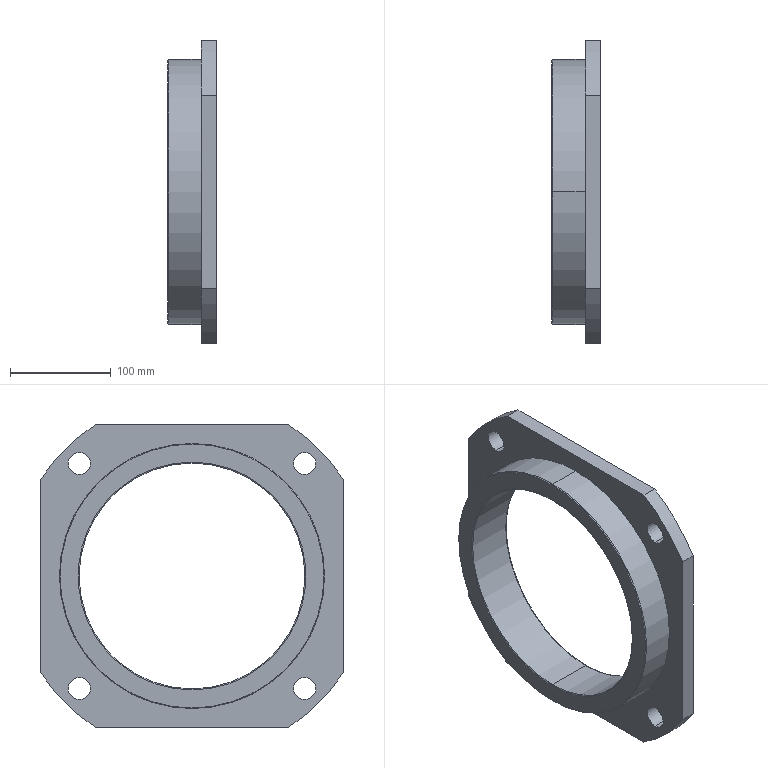Part | SolidWorks | features Chamfer 3, ICE 2, CirPattern 1, RefAxis 1, Revolution 1 | 1 solid | 29 faces | box 48 x 300 x 300 mm | volume 1152473 mm3 | cylinder 16 | plane 7 | cone 6 | commonest cylinder face diameters 22 x8 356 x4 224 x2 263 x2
STEP:
#1=CARTESIAN_POINT('',(-36.947,0.,130.923));
#2=VERTEX_POINT('',#1);
#3=CARTESIAN_POINT('',(-36.947,0.,-130.923));
#4=VERTEX_POINT('',#3);
#5=CARTESIAN_POINT('',(-36.947,0.,0.));
#6=DIRECTION('',(-1.,0.,0.));
#7=DIRECTION('',(0.,0.,-1.));
#8=AXIS2_PLACEMENT_3D('',#5,#6,#7);
#9=CIRCLE('',#8,130.923);
#10=EDGE_CURVE('',#2,#4,#9,.T.);
#11=ORIENTED_EDGE('',*,*,#10,.F.);
#12=CARTESIAN_POINT('',(-35.947,0.,131.5));
#13=VERTEX_POINT('',#12);
#14=CARTESIAN_POINT('',(-36.947,0.,130.923));
#15=DIRECTION('',(0.866,0.,0.5));
#16=VECTOR('',#15,1000.);
#17=LINE('',#14,#16);
#18=EDGE_CURVE('',#2,#13,#17,.T.);
#19=ORIENTED_EDGE('',*,*,#18,.T.);
#20=CARTESIAN_POINT('',(-35.947,0.,-131.5));
#21=VERTEX_POINT('',#20);
#22=CARTESIAN_POINT('',(-35.947,0.,0.));
#23=DIRECTION('',(1.,0.,0.));
#24=DIRECTION('',(0.,0.,-1.));
#25=AXIS2_PLACEMENT_3D('',#22,#23,#24);
#26=CIRCLE('',#25,131.5);
#27=EDGE_CURVE('',#21,#13,#26,.T.);
#28=ORIENTED_EDGE('',*,*,#27,.F.);
#29=CARTESIAN_POINT('',(-36.947,0.,-130.923));
#30=DIRECTION('',(0.866,0.,-0.5));
#31=VECTOR('',#30,1000.);
#32=LINE('',#29,#31);
#33=EDGE_CURVE('',#4,#21,#32,.T.);
#34=ORIENTED_EDGE('',*,*,#33,.F.);
#35=EDGE_LOOP('',(#11,#19,#28,#34));
#36=FACE_OUTER_BOUND('',#35,.T.);
#37=CARTESIAN_POINT('',(-36.947,0.,0.));
#38=DIRECTION('',(1.,0.,0.));
#39=DIRECTION('',(0.,0.,-1.));
#40=AXIS2_PLACEMENT_3D('',#37,#38,#39);
#41=CONICAL_SURFACE('',#40,130.923,0.5236);
#42=ADVANCED_FACE('',(#36),#41,.T.);
#43=CARTESIAN_POINT('',(-36.37,0.,-112.));
#44=VERTEX_POINT('',#43);
#45=CARTESIAN_POINT('',(-36.37,0.,112.));
#46=VERTEX_POINT('',#45);
#47=CARTESIAN_POINT('',(-36.37,0.,0.));
#48=DIRECTION('',(-1.,0.,0.));
#49=DIRECTION('',(0.,0.,-1.));
#50=AXIS2_PLACEMENT_3D('',#47,#48,#49);
#51=CIRCLE('',#50,112.);
#52=EDGE_CURVE('',#44,#46,#51,.T.);
#53=ORIENTED_EDGE('',*,*,#52,.F.);
#54=CARTESIAN_POINT('',(-36.947,0.,-113.));
#55=VERTEX_POINT('',#54);
#56=CARTESIAN_POINT('',(-36.37,0.,-112.));
#57=DIRECTION('',(-0.5,0.,-0.866));
#58=VECTOR('',#57,1000.);
#59=LINE('',#56,#58);
#60=EDGE_CURVE('',#44,#55,#59,.T.);
#61=ORIENTED_EDGE('',*,*,#60,.T.);
#62=CARTESIAN_POINT('',(-36.947,0.,113.));
#63=VERTEX_POINT('',#62);
#64=CARTESIAN_POINT('',(-36.947,0.,0.));
#65=DIRECTION('',(1.,0.,0.));
#66=DIRECTION('',(0.,0.,-1.));
#67=AXIS2_PLACEMENT_3D('',#64,#65,#66);
#68=CIRCLE('',#67,113.);
#69=EDGE_CURVE('',#63,#55,#68,.T.);
#70=ORIENTED_EDGE('',*,*,#69,.F.);
#71=CARTESIAN_POINT('',(-36.37,0.,112.));
#72=DIRECTION('',(-0.5,0.,0.866));
#73=VECTOR('',#72,1000.);
#74=LINE('',#71,#73);
#75=EDGE_CURVE('',#46,#63,#74,.T.);
#76=ORIENTED_EDGE('',*,*,#75,.F.);
#77=EDGE_LOOP('',(#53,#61,#70,#76));
#78=FACE_OUTER_BOUND('',#77,.T.);
#79=CARTESIAN_POINT('',(-36.37,0.,0.));
#80=DIRECTION('',(-1.,0.,0.));
#81=DIRECTION('',(0.,0.,1.));
#82=AXIS2_PLACEMENT_3D('',#79,#80,#81);
#83=CONICAL_SURFACE('',#82,112.,1.047);
#84=ADVANCED_FACE('',(#78),#83,.F.);
#85=CARTESIAN_POINT('',(10.053,0.,112.));
#86=VERTEX_POINT('',#85);
#87=CARTESIAN_POINT('',(10.053,0.,-112.));
#88=VERTEX_POINT('',#87);
#89=CARTESIAN_POINT('',(10.053,0.,0.));
#90=DIRECTION('',(1.,0.,0.));
#91=DIRECTION('',(0.,0.,1.));
#92=AXIS2_PLACEMENT_3D('',#89,#90,#91);
#93=CIRCLE('',#92,112.);
#94=EDGE_CURVE('',#86,#88,#93,.T.);
#95=ORIENTED_EDGE('',*,*,#94,.F.);
#96=CARTESIAN_POINT('',(11.053,0.,112.577));
#97=VERTEX_POINT('',#96);
#98=CARTESIAN_POINT('',(11.053,0.,112.577));
#99=DIRECTION('',(0.866,0.,0.5));
#100=VECTOR('',#99,1000.);
#101=LINE('',#98,#100);
#102=EDGE_CURVE('',#86,#97,#101,.T.);
#103=ORIENTED_EDGE('',*,*,#102,.T.);
#104=CARTESIAN_POINT('',(11.053,0.,-112.577));
#105=VERTEX_POINT('',#104);
#106=CARTESIAN_POINT('',(11.053,0.,0.));
#107=DIRECTION('',(-1.,0.,0.));
#108=DIRECTION('',(0.,0.,1.));
#109=AXIS2_PLACEMENT_3D('',#106,#107,#108);
#110=CIRCLE('',#109,112.577);
#111=EDGE_CURVE('',#105,#97,#110,.T.);
#112=ORIENTED_EDGE('',*,*,#111,.F.);
#113=CARTESIAN_POINT('',(11.053,0.,-112.577));
#114=DIRECTION('',(0.866,0.,-0.5));
#115=VECTOR('',#114,1000.);
#116=LINE('',#113,#115);
#117=EDGE_CURVE('',#88,#105,#116,.T.);
#118=ORIENTED_EDGE('',*,*,#117,.F.);
#119=EDGE_LOOP('',(#95,#103,#112,#118));
#120=FACE_OUTER_BOUND('',#119,.T.);
#121=CARTESIAN_POINT('',(11.053,0.,0.));
#122=DIRECTION('',(1.,0.,0.));
#123=DIRECTION('',(0.,0.,-1.));
#124=AXIS2_PLACEMENT_3D('',#121,#122,#123);
#125=CONICAL_SURFACE('',#124,112.577,0.5236);
#126=ADVANCED_FACE('',(#120),#125,.F.);
#127=CARTESIAN_POINT('',(-3.947,111.723,122.723));
#128=VERTEX_POINT('',#127);
#129=CARTESIAN_POINT('',(-3.947,111.723,100.723));
#130=VERTEX_POINT('',#129);
#131=CARTESIAN_POINT('',(-3.947,111.723,111.723));
#132=DIRECTION('',(1.,0.,0.));
#133=DIRECTION('',(0.,1.,0.));
#134=AXIS2_PLACEMENT_3D('',#131,#132,#133);
#135=CIRCLE('',#134,11.);
#136=EDGE_CURVE('',#128,#130,#135,.T.);
#137=ORIENTED_EDGE('',*,*,#136,.F.);
#138=CARTESIAN_POINT('',(11.053,111.723,122.723));
#139=VERTEX_POINT('',#138);
#140=CARTESIAN_POINT('',(-3.947,111.723,122.723));
#141=DIRECTION('',(1.,0.,0.));
#142=VECTOR('',#141,1000.);
#143=LINE('',#140,#142);
#144=EDGE_CURVE('',#128,#139,#143,.T.);
#145=ORIENTED_EDGE('',*,*,#144,.T.);
#146=CARTESIAN_POINT('',(11.053,111.723,100.723));
#147=VERTEX_POINT('',#146);
#148=CARTESIAN_POINT('',(11.053,111.723,111.723));
#149=DIRECTION('',(1.,0.,0.));
#150=DIRECTION('',(0.,1.,0.));
#151=AXIS2_PLACEMENT_3D('',#148,#149,#150);
#152=CIRCLE('',#151,11.);
#153=EDGE_CURVE('',#139,#147,#152,.T.);
#154=ORIENTED_EDGE('',*,*,#153,.T.);
#155=CARTESIAN_POINT('',(-3.947,111.723,100.723));
#156=DIRECTION('',(1.,0.,0.));
#157=VECTOR('',#156,1000.);
#158=LINE('',#155,#157);
#159=EDGE_CURVE('',#130,#147,#158,.T.);
#160=ORIENTED_EDGE('',*,*,#159,.F.);
#161=EDGE_LOOP('',(#137,#145,#154,#160));
#162=FACE_OUTER_BOUND('',#161,.T.);
#163=CARTESIAN_POINT('',(-3.947,111.723,111.723));
#164=DIRECTION('',(1.,0.,0.));
#165=DIRECTION('',(0.,0.,-1.));
#166=AXIS2_PLACEMENT_3D('',#163,#164,#165);
#167=CYLINDRICAL_SURFACE('',#166,11.);
#168=ADVANCED_FACE('',(#162),#167,.F.);
#169=CARTESIAN_POINT('',(-3.947,-111.723,122.723));
#170=VERTEX_POINT('',#169);
#171=CARTESIAN_POINT('',(-3.947,-111.723,100.723));
#172=VERTEX_POINT('',#171);
#173=CARTESIAN_POINT('',(-3.947,-111.723,111.723));
#174=DIRECTION('',(1.,0.,0.));
#175=DIRECTION('',(0.,0.,1.));
#176=AXIS2_PLACEMENT_3D('',#173,#174,#175);
#177=CIRCLE('',#176,11.);
#178=EDGE_CURVE('',#170,#172,#177,.T.);
#179=ORIENTED_EDGE('',*,*,#178,.F.);
#180=CARTESIAN_POINT('',(11.053,-111.723,122.723));
#181=VERTEX_POINT('',#180);
#182=CARTESIAN_POINT('',(-3.947,-111.723,122.723));
#183=DIRECTION('',(1.,0.,0.));
#184=VECTOR('',#183,1000.);
#185=LINE('',#182,#184);
#186=EDGE_CURVE('',#170,#181,#185,.T.);
#187=ORIENTED_EDGE('',*,*,#186,.T.);
#188=CARTESIAN_POINT('',(11.053,-111.723,100.723));
#189=VERTEX_POINT('',#188);
#190=CARTESIAN_POINT('',(11.053,-111.723,111.723));
#191=DIRECTION('',(1.,0.,0.));
#192=DIRECTION('',(0.,0.,1.));
#193=AXIS2_PLACEMENT_3D('',#190,#191,#192);
#194=CIRCLE('',#193,11.);
#195=EDGE_CURVE('',#181,#189,#194,.T.);
#196=ORIENTED_EDGE('',*,*,#195,.T.);
#197=CARTESIAN_POINT('',(-3.947,-111.723,100.723));
#198=DIRECTION('',(1.,0.,0.));
#199=VECTOR('',#198,1000.);
#200=LINE('',#197,#199);
#201=EDGE_CURVE('',#172,#189,#200,.T.);
#202=ORIENTED_EDGE('',*,*,#201,.F.);
#203=EDGE_LOOP('',(#179,#187,#196,#202));
#204=FACE_OUTER_BOUND('',#203,.T.);
#205=CARTESIAN_POINT('',(-3.947,-111.723,111.723));
#206=DIRECTION('',(1.,0.,0.));
#207=DIRECTION('',(0.,0.,-1.));
#208=AXIS2_PLACEMENT_3D('',#205,#206,#207);
#209=CYLINDRICAL_SURFACE('',#208,11.);
#210=ADVANCED_FACE('',(#204),#209,.F.);
#211=CARTESIAN_POINT('',(-3.947,-111.723,-100.723));
#212=VERTEX_POINT('',#211);
#213=CARTESIAN_POINT('',(-3.947,-111.723,-122.723));
#214=VERTEX_POINT('',#213);
#215=CARTESIAN_POINT('',(-3.947,-111.723,-111.723));
#216=DIRECTION('',(1.,0.,0.));
#217=DIRECTION('',(0.,-1.,0.));
#218=AXIS2_PLACEMENT_3D('',#215,#216,#217);
#219=CIRCLE('',#218,11.);
#220=EDGE_CURVE('',#212,#214,#219,.T.);
#221=ORIENTED_EDGE('',*,*,#220,.F.);
#222=CARTESIAN_POINT('',(11.053,-111.723,-100.723));
#223=VERTEX_POINT('',#222);
#224=CARTESIAN_POINT('',(-3.947,-111.723,-100.723));
#225=DIRECTION('',(1.,0.,0.));
#226=VECTOR('',#225,1000.);
#227=LINE('',#224,#226);
#228=EDGE_CURVE('',#212,#223,#227,.T.);
#229=ORIENTED_EDGE('',*,*,#228,.T.);
#230=CARTESIAN_POINT('',(11.053,-111.723,-122.723));
#231=VERTEX_POINT('',#230);
#232=CARTESIAN_POINT('',(11.053,-111.723,-111.723));
#233=DIRECTION('',(1.,0.,0.));
#234=DIRECTION('',(0.,-1.,0.));
#235=AXIS2_PLACEMENT_3D('',#232,#233,#234);
#236=CIRCLE('',#235,11.);
#237=EDGE_CURVE('',#223,#231,#236,.T.);
#238=ORIENTED_EDGE('',*,*,#237,.T.);
#239=CARTESIAN_POINT('',(-3.947,-111.723,-122.723));
#240=DIRECTION('',(1.,0.,0.));
#241=VECTOR('',#240,1000.);
#242=LINE('',#239,#241);
#243=EDGE_CURVE('',#214,#231,#242,.T.);
#244=ORIENTED_EDGE('',*,*,#243,.F.);
#245=EDGE_LOOP('',(#221,#229,#238,#244));
#246=FACE_OUTER_BOUND('',#245,.T.);
#247=CARTESIAN_POINT('',(-3.947,-111.723,-111.723));
#248=DIRECTION('',(1.,0.,0.));
#249=DIRECTION('',(0.,0.,-1.));
#250=AXIS2_PLACEMENT_3D('',#247,#248,#249);
#251=CYLINDRICAL_SURFACE('',#250,11.);
#252=ADVANCED_FACE('',(#246),#251,.F.);
#253=CARTESIAN_POINT('',(-3.947,111.723,-100.723));
#254=VERTEX_POINT('',#253);
#255=CARTESIAN_POINT('',(-3.947,111.723,-122.723));
#256=VERTEX_POINT('',#255);
#257=CARTESIAN_POINT('',(-3.947,111.723,-111.723));
#258=DIRECTION('',(1.,0.,0.));
#259=DIRECTION('',(0.,0.,-1.));
#260=AXIS2_PLACEMENT_3D('',#257,#258,#259);
#261=CIRCLE('',#260,11.);
#262=EDGE_CURVE('',#254,#256,#261,.T.);
#263=ORIENTED_EDGE('',*,*,#262,.F.);
#264=CARTESIAN_POINT('',(11.053,111.723,-100.723));
#265=VERTEX_POINT('',#264);
#266=CARTESIAN_POINT('',(-3.947,111.723,-100.723));
#267=DIRECTION('',(1.,0.,0.));
#268=VECTOR('',#267,1000.);
#269=LINE('',#266,#268);
#270=EDGE_CURVE('',#254,#265,#269,.T.);
#271=ORIENTED_EDGE('',*,*,#270,.T.);
#272=CARTESIAN_POINT('',(11.053,111.723,-122.723));
#273=VERTEX_POINT('',#272);
#274=CARTESIAN_POINT('',(11.053,111.723,-111.723));
#275=DIRECTION('',(1.,0.,0.));
#276=DIRECTION('',(0.,0.,-1.));
#277=AXIS2_PLACEMENT_3D('',#274,#275,#276);
#278=CIRCLE('',#277,11.);
#279=EDGE_CURVE('',#265,#273,#278,.T.);
#280=ORIENTED_EDGE('',*,*,#279,.T.);
#281=CARTESIAN_POINT('',(-3.947,111.723,-122.723));
#282=DIRECTION('',(1.,0.,0.));
#283=VECTOR('',#282,1000.);
#284=LINE('',#281,#283);
#285=EDGE_CURVE('',#256,#273,#284,.T.);
#286=ORIENTED_EDGE('',*,*,#285,.F.);
#287=EDGE_LOOP('',(#263,#271,#280,#286));
#288=FACE_OUTER_BOUND('',#287,.T.);
#289=CARTESIAN_POINT('',(-3.947,111.723,-111.723));
#290=DIRECTION('',(1.,0.,0.));
#291=DIRECTION('',(0.,0.,-1.));
#292=AXIS2_PLACEMENT_3D('',#289,#290,#291);
#293=CYLINDRICAL_SURFACE('',#292,11.);
#294=ADVANCED_FACE('',(#288),#293,.F.);
#295=ORIENTED_EDGE('',*,*,#94,.T.);
#296=CARTESIAN_POINT('',(-77.414,0.,-112.));
#297=DIRECTION('',(-1.,0.,0.));
#298=VECTOR('',#297,1000.);
#299=LINE('',#296,#298);
#300=EDGE_CURVE('',#88,#44,#299,.T.);
#301=ORIENTED_EDGE('',*,*,#300,.T.);
#302=ORIENTED_EDGE('',*,*,#52,.T.);
#303=CARTESIAN_POINT('',(-77.414,0.,112.));
#304=DIRECTION('',(-1.,0.,0.));
#305=VECTOR('',#304,1000.);
#306=LINE('',#303,#305);
#307=EDGE_CURVE('',#86,#46,#306,.T.);
#308=ORIENTED_EDGE('',*,*,#307,.F.);
#309=EDGE_LOOP('',(#295,#301,#302,#308));
#310=FACE_OUTER_BOUND('',#309,.T.);
#311=CARTESIAN_POINT('',(-77.414,0.,0.));
#312=DIRECTION('',(-1.,0.,0.));
#313=DIRECTION('',(0.,0.,1.));
#314=AXIS2_PLACEMENT_3D('',#311,#312,#313);
#315=CYLINDRICAL_SURFACE('',#314,112.);
#316=ADVANCED_FACE('',(#310),#315,.F.);
#317=CARTESIAN_POINT('',(-3.947,0.,131.5));
#318=VERTEX_POINT('',#317);
#319=CARTESIAN_POINT('',(-3.947,0.,-131.5));
#320=VERTEX_POINT('',#319);
#321=CARTESIAN_POINT('',(-3.947,0.,0.));
#322=DIRECTION('',(-1.,0.,0.));
#323=DIRECTION('',(0.,0.,1.));
#324=AXIS2_PLACEMENT_3D('',#321,#322,#323);
#325=CIRCLE('',#324,131.5);
#326=EDGE_CURVE('',#318,#320,#325,.T.);
#327=ORIENTED_EDGE('',*,*,#326,.T.);
#328=CARTESIAN_POINT('',(-77.414,0.,-131.5));
#329=DIRECTION('',(-1.,0.,0.));
#330=VECTOR('',#329,1000.);
#331=LINE('',#328,#330);
#332=EDGE_CURVE('',#320,#21,#331,.T.);
#333=ORIENTED_EDGE('',*,*,#332,.T.);
#334=ORIENTED_EDGE('',*,*,#27,.T.);
#335=CARTESIAN_POINT('',(-77.414,0.,131.5));
#336=DIRECTION('',(-1.,0.,0.));
#337=VECTOR('',#336,1000.);
#338=LINE('',#335,#337);
#339=EDGE_CURVE('',#318,#13,#338,.T.);
#340=ORIENTED_EDGE('',*,*,#339,.F.);
#341=EDGE_LOOP('',(#327,#333,#334,#340));
#342=FACE_OUTER_BOUND('',#341,.T.);
#343=CARTESIAN_POINT('',(-77.414,0.,0.));
#344=DIRECTION('',(-1.,0.,0.));
#345=DIRECTION('',(0.,0.,1.));
#346=AXIS2_PLACEMENT_3D('',#343,#344,#345);
#347=CYLINDRICAL_SURFACE('',#346,131.5);
#348=ADVANCED_FACE('',(#342),#347,.T.);
#349=CARTESIAN_POINT('',(11.053,-150.,95.833));
#350=VERTEX_POINT('',#349);
#351=CARTESIAN_POINT('',(11.053,-95.833,150.));
#352=VERTEX_POINT('',#351);
#353=CARTESIAN_POINT('',(11.053,0.,0.));
#354=DIRECTION('',(-1.,0.,0.));
#355=DIRECTION('',(0.,0.,1.));
#356=AXIS2_PLACEMENT_3D('',#353,#354,#355);
#357=CIRCLE('',#356,178.);
#358=EDGE_CURVE('',#350,#352,#357,.T.);
#359=ORIENTED_EDGE('',*,*,#358,.T.);
#360=CARTESIAN_POINT('',(-3.947,-95.833,150.));
#361=VERTEX_POINT('',#360);
#362=CARTESIAN_POINT('',(-3.947,-95.833,150.));
#363=DIRECTION('',(1.,0.,0.));
#364=VECTOR('',#363,1000.);
#365=LINE('',#362,#364);
#366=EDGE_CURVE('',#361,#352,#365,.T.);
#367=ORIENTED_EDGE('',*,*,#366,.F.);
#368=CARTESIAN_POINT('',(-3.947,-150.,95.833));
#369=VERTEX_POINT('',#368);
#370=CARTESIAN_POINT('',(-3.947,0.,0.));
#371=DIRECTION('',(-1.,0.,0.));
#372=DIRECTION('',(0.,0.,1.));
#373=AXIS2_PLACEMENT_3D('',#370,#371,#372);
#374=CIRCLE('',#373,178.);
#375=EDGE_CURVE('',#369,#361,#374,.T.);
#376=ORIENTED_EDGE('',*,*,#375,.F.);
#377=CARTESIAN_POINT('',(-3.947,-150.,95.833));
#378=DIRECTION('',(1.,0.,0.));
#379=VECTOR('',#378,1000.);
#380=LINE('',#377,#379);
#381=EDGE_CURVE('',#369,#350,#380,.T.);
#382=ORIENTED_EDGE('',*,*,#381,.T.);
#383=EDGE_LOOP('',(#359,#367,#376,#382));
#384=FACE_OUTER_BOUND('',#383,.T.);
#385=CARTESIAN_POINT('',(-77.414,0.,0.));
#386=DIRECTION('',(-1.,0.,0.));
#387=DIRECTION('',(0.,0.,1.));
#388=AXIS2_PLACEMENT_3D('',#385,#386,#387);
#389=CYLINDRICAL_SURFACE('',#388,178.);
#390=ADVANCED_FACE('',(#384),#389,.T.);
#391=CARTESIAN_POINT('',(-3.947,95.833,150.));
#392=VERTEX_POINT('',#391);
#393=CARTESIAN_POINT('',(-3.947,150.,95.833));
#394=VERTEX_POINT('',#393);
#395=CARTESIAN_POINT('',(-3.947,0.,0.));
#396=DIRECTION('',(-1.,0.,0.));
#397=DIRECTION('',(0.,0.,1.));
#398=AXIS2_PLACEMENT_3D('',#395,#396,#397);
#399=CIRCLE('',#398,178.);
#400=EDGE_CURVE('',#392,#394,#399,.T.);
#401=ORIENTED_EDGE('',*,*,#400,.F.);
#402=CARTESIAN_POINT('',(11.053,95.833,150.));
#403=VERTEX_POINT('',#402);
#404=CARTESIAN_POINT('',(-3.947,95.833,150.));
#405=DIRECTION('',(1.,0.,0.));
#406=VECTOR('',#405,1000.);
#407=LINE('',#404,#406);
#408=EDGE_CURVE('',#392,#403,#407,.T.);
#409=ORIENTED_EDGE('',*,*,#408,.T.);
#410=CARTESIAN_POINT('',(11.053,150.,95.833));
#411=VERTEX_POINT('',#410);
#412=CARTESIAN_POINT('',(11.053,0.,0.));
#413=DIRECTION('',(-1.,0.,0.));
#414=DIRECTION('',(0.,0.,1.));
#415=AXIS2_PLACEMENT_3D('',#412,#413,#414);
#416=CIRCLE('',#415,178.);
#417=EDGE_CURVE('',#403,#411,#416,.T.);
#418=ORIENTED_EDGE('',*,*,#417,.T.);
#419=CARTESIAN_POINT('',(-3.947,150.,95.833));
#420=DIRECTION('',(1.,0.,0.));
#421=VECTOR('',#420,1000.);
#422=LINE('',#419,#421);
#423=EDGE_CURVE('',#394,#411,#422,.T.);
#424=ORIENTED_EDGE('',*,*,#423,.F.);
#425=EDGE_LOOP('',(#401,#409,#418,#424));
#426=FACE_OUTER_BOUND('',#425,.T.);
#427=CARTESIAN_POINT('',(-77.414,0.,0.));
#428=DIRECTION('',(-1.,0.,0.));
#429=DIRECTION('',(0.,0.,1.));
#430=AXIS2_PLACEMENT_3D('',#427,#428,#429);
#431=CYLINDRICAL_SURFACE('',#430,178.);
#432=ADVANCED_FACE('',(#426),#431,.T.);
#433=CARTESIAN_POINT('',(11.053,-95.833,-150.));
#434=VERTEX_POINT('',#433);
#435=CARTESIAN_POINT('',(11.053,-150.,-95.833));
#436=VERTEX_POINT('',#435);
#437=CARTESIAN_POINT('',(11.053,0.,0.));
#438=DIRECTION('',(-1.,0.,0.));
#439=DIRECTION('',(0.,0.,1.));
#440=AXIS2_PLACEMENT_3D('',#437,#438,#439);
#441=CIRCLE('',#440,178.);
#442=EDGE_CURVE('',#434,#436,#441,.T.);
#443=ORIENTED_EDGE('',*,*,#442,.T.);
#444=CARTESIAN_POINT('',(-3.947,-150.,-95.833));
#445=VERTEX_POINT('',#444);
#446=CARTESIAN_POINT('',(-3.947,-150.,-95.833));
#447=DIRECTION('',(1.,0.,0.));
#448=VECTOR('',#447,1000.);
#449=LINE('',#446,#448);
#450=EDGE_CURVE('',#445,#436,#449,.T.);
#451=ORIENTED_EDGE('',*,*,#450,.F.);
#452=CARTESIAN_POINT('',(-3.947,-95.833,-150.));
#453=VERTEX_POINT('',#452);
#454=CARTESIAN_POINT('',(-3.947,0.,0.));
#455=DIRECTION('',(-1.,0.,0.));
#456=DIRECTION('',(0.,0.,1.));
#457=AXIS2_PLACEMENT_3D('',#454,#455,#456);
#458=CIRCLE('',#457,178.);
#459=EDGE_CURVE('',#453,#445,#458,.T.);
#460=ORIENTED_EDGE('',*,*,#459,.F.);
#461=CARTESIAN_POINT('',(-3.947,-95.833,-150.));
#462=DIRECTION('',(1.,0.,0.));
#463=VECTOR('',#462,1000.);
#464=LINE('',#461,#463);
#465=EDGE_CURVE('',#453,#434,#464,.T.);
#466=ORIENTED_EDGE('',*,*,#465,.T.);
#467=EDGE_LOOP('',(#443,#451,#460,#466));
#468=FACE_OUTER_BOUND('',#467,.T.);
#469=CARTESIAN_POINT('',(-77.414,0.,0.));
#470=DIRECTION('',(-1.,0.,0.));
#471=DIRECTION('',(0.,0.,1.));
#472=AXIS2_PLACEMENT_3D('',#469,#470,#471);
#473=CYLINDRICAL_SURFACE('',#472,178.);
#474=ADVANCED_FACE('',(#468),#473,.T.);
#475=CARTESIAN_POINT('',(-36.947,0.,0.));
#476=DIRECTION('',(-1.,0.,0.));
#477=DIRECTION('',(0.,0.,-1.));
#478=AXIS2_PLACEMENT_3D('',#475,#476,#477);
#479=CIRCLE('',#478,130.923);
#480=EDGE_CURVE('',#4,#2,#479,.T.);
#481=ORIENTED_EDGE('',*,*,#480,.T.);
#482=ORIENTED_EDGE('',*,*,#10,.T.);
#483=EDGE_LOOP('',(#481,#482));
#484=FACE_OUTER_BOUND('',#483,.T.);
#485=ORIENTED_EDGE('',*,*,#69,.T.);
#486=CARTESIAN_POINT('',(-36.947,0.,0.));
#487=DIRECTION('',(1.,0.,0.));
#488=DIRECTION('',(0.,0.,-1.));
#489=AXIS2_PLACEMENT_3D('',#486,#487,#488);
#490=CIRCLE('',#489,113.);
#491=EDGE_CURVE('',#55,#63,#490,.T.);
#492=ORIENTED_EDGE('',*,*,#491,.T.);
#493=EDGE_LOOP('',(#485,#492));
#494=FACE_BOUND('',#493,.T.);
#495=CARTESIAN_POINT('',(-36.947,112.,0.));
#496=DIRECTION('',(1.,0.,0.));
#497=DIRECTION('',(0.,0.,-1.));
#498=AXIS2_PLACEMENT_3D('',#495,#496,#497);
#499=PLANE('',#498);
#500=ADVANCED_FACE('',(#484,#494),#499,.F.);
#501=ORIENTED_EDGE('',*,*,#332,.F.);
#502=CARTESIAN_POINT('',(-3.947,0.,0.));
#503=DIRECTION('',(-1.,0.,0.));
#504=DIRECTION('',(0.,0.,1.));
#505=AXIS2_PLACEMENT_3D('',#502,#503,#504);
#506=CIRCLE('',#505,131.5);
#507=EDGE_CURVE('',#320,#318,#506,.T.);
#508=ORIENTED_EDGE('',*,*,#507,.T.);
#509=ORIENTED_EDGE('',*,*,#339,.T.);
#510=CARTESIAN_POINT('',(-35.947,0.,0.));
#511=DIRECTION('',(1.,0.,0.));
#512=DIRECTION('',(0.,0.,-1.));
#513=AXIS2_PLACEMENT_3D('',#510,#511,#512);
#514=CIRCLE('',#513,131.5);
#515=EDGE_CURVE('',#13,#21,#514,.T.);
#516=ORIENTED_EDGE('',*,*,#515,.T.);
#517=EDGE_LOOP('',(#501,#508,#509,#516));
#518=FACE_OUTER_BOUND('',#517,.T.);
#519=CARTESIAN_POINT('',(-77.414,0.,0.));
#520=DIRECTION('',(-1.,0.,0.));
#521=DIRECTION('',(0.,0.,1.));
#522=AXIS2_PLACEMENT_3D('',#519,#520,#521);
#523=CYLINDRICAL_SURFACE('',#522,131.5);
#524=ADVANCED_FACE('',(#518),#523,.T.);
#525=CARTESIAN_POINT('',(-3.947,111.723,111.723));
#526=DIRECTION('',(1.,0.,0.));
#527=DIRECTION('',(0.,1.,0.));
#528=AXIS2_PLACEMENT_3D('',#525,#526,#527);
#529=CIRCLE('',#528,11.);
#530=EDGE_CURVE('',#130,#128,#529,.T.);
#531=ORIENTED_EDGE('',*,*,#530,.T.);
#532=ORIENTED_EDGE('',*,*,#136,.T.);
#533=EDGE_LOOP('',(#531,#532));
#534=FACE_BOUND('',#533,.T.);
#535=CARTESIAN_POINT('',(-3.947,-111.723,111.723));
#536=DIRECTION('',(1.,0.,0.));
#537=DIRECTION('',(0.,0.,1.));
#538=AXIS2_PLACEMENT_3D('',#535,#536,#537);
#539=CIRCLE('',#538,11.);
#540=EDGE_CURVE('',#172,#170,#539,.T.);
#541=ORIENTED_EDGE('',*,*,#540,.T.);
#542=ORIENTED_EDGE('',*,*,#178,.T.);
#543=EDGE_LOOP('',(#541,#542));
#544=FACE_BOUND('',#543,.T.);
#545=CARTESIAN_POINT('',(-3.947,-111.723,-111.723));
#546=DIRECTION('',(1.,0.,0.));
#547=DIRECTION('',(0.,-1.,0.));
#548=AXIS2_PLACEMENT_3D('',#545,#546,#547);
#549=CIRCLE('',#548,11.);
#550=EDGE_CURVE('',#214,#212,#549,.T.);
#551=ORIENTED_EDGE('',*,*,#550,.T.);
#552=ORIENTED_EDGE('',*,*,#220,.T.);
#553=EDGE_LOOP('',(#551,#552));
#554=FACE_BOUND('',#553,.T.);
#555=CARTESIAN_POINT('',(-3.947,111.723,-111.723));
#556=DIRECTION('',(1.,0.,0.));
#557=DIRECTION('',(0.,0.,-1.));
#558=AXIS2_PLACEMENT_3D('',#555,#556,#557);
#559=CIRCLE('',#558,11.);
#560=EDGE_CURVE('',#256,#254,#559,.T.);
#561=ORIENTED_EDGE('',*,*,#560,.T.);
#562=ORIENTED_EDGE('',*,*,#262,.T.);
#563=EDGE_LOOP('',(#561,#562));
#564=FACE_BOUND('',#563,.T.);
#565=ORIENTED_EDGE('',*,*,#326,.F.);
#566=ORIENTED_EDGE('',*,*,#507,.F.);
#567=EDGE_LOOP('',(#565,#566));
#568=FACE_BOUND('',#567,.T.);
#569=ORIENTED_EDGE('',*,*,#375,.T.);
#570=CARTESIAN_POINT('',(-3.947,95.833,150.));
#571=DIRECTION('',(0.,1.,0.));
#572=VECTOR('',#571,1000.);
#573=LINE('',#570,#572);
#574=EDGE_CURVE('',#361,#392,#573,.T.);
#575=ORIENTED_EDGE('',*,*,#574,.T.);
#576=ORIENTED_EDGE('',*,*,#400,.T.);
#577=CARTESIAN_POINT('',(-3.947,150.,-95.833));
#578=VERTEX_POINT('',#577);
#579=CARTESIAN_POINT('',(-3.947,150.,95.833));
#580=DIRECTION('',(0.,0.,-1.));
#581=VECTOR('',#580,1000.);
#582=LINE('',#579,#581);
#583=EDGE_CURVE('',#394,#578,#582,.T.);
#584=ORIENTED_EDGE('',*,*,#583,.T.);
#585=CARTESIAN_POINT('',(-3.947,95.833,-150.));
#586=VERTEX_POINT('',#585);
#587=CARTESIAN_POINT('',(-3.947,0.,0.));
#588=DIRECTION('',(-1.,0.,0.));
#589=DIRECTION('',(0.,0.,1.));
#590=AXIS2_PLACEMENT_3D('',#587,#588,#589);
#591=CIRCLE('',#590,178.);
#592=EDGE_CURVE('',#578,#586,#591,.T.);
#593=ORIENTED_EDGE('',*,*,#592,.T.);
#594=CARTESIAN_POINT('',(-3.947,95.833,-150.));
#595=DIRECTION('',(0.,-1.,0.));
#596=VECTOR('',#595,1000.);
#597=LINE('',#594,#596);
#598=EDGE_CURVE('',#586,#453,#597,.T.);
#599=ORIENTED_EDGE('',*,*,#598,.T.);
#600=ORIENTED_EDGE('',*,*,#459,.T.);
#601=CARTESIAN_POINT('',(-3.947,-150.,95.833));
#602=DIRECTION('',(0.,0.,1.));
#603=VECTOR('',#602,1000.);
#604=LINE('',#601,#603);
#605=EDGE_CURVE('',#445,#369,#604,.T.);
#606=ORIENTED_EDGE('',*,*,#605,.T.);
#607=EDGE_LOOP('',(#569,#575,#576,#584,#593,#599,#600,#606));
#608=FACE_OUTER_BOUND('',#607,.T.);
#609=CARTESIAN_POINT('',(-3.947,131.5,0.));
#610=DIRECTION('',(1.,0.,0.));
#611=DIRECTION('',(0.,0.,-1.));
#612=AXIS2_PLACEMENT_3D('',#609,#610,#611);
#613=PLANE('',#612);
#614=ADVANCED_FACE('',(#534,#544,#554,#564,#568,#608),#613,.F.);
#615=ORIENTED_EDGE('',*,*,#592,.F.);
#616=CARTESIAN_POINT('',(11.053,150.,-95.833));
#617=VERTEX_POINT('',#616);
#618=CARTESIAN_POINT('',(-3.947,150.,-95.833));
#619=DIRECTION('',(1.,0.,0.));
#620=VECTOR('',#619,1000.);
#621=LINE('',#618,#620);
#622=EDGE_CURVE('',#578,#617,#621,.T.);
#623=ORIENTED_EDGE('',*,*,#622,.T.);
#624=CARTESIAN_POINT('',(11.053,95.833,-150.));
#625=VERTEX_POINT('',#624);
#626=CARTESIAN_POINT('',(11.053,0.,0.));
#627=DIRECTION('',(-1.,0.,0.));
#628=DIRECTION('',(0.,0.,1.));
#629=AXIS2_PLACEMENT_3D('',#626,#627,#628);
#630=CIRCLE('',#629,178.);
#631=EDGE_CURVE('',#617,#625,#630,.T.);
#632=ORIENTED_EDGE('',*,*,#631,.T.);
#633=CARTESIAN_POINT('',(-3.947,95.833,-150.));
#634=DIRECTION('',(1.,0.,0.));
#635=VECTOR('',#634,1000.);
#636=LINE('',#633,#635);
#637=EDGE_CURVE('',#586,#625,#636,.T.);
#638=ORIENTED_EDGE('',*,*,#637,.F.);
#639=EDGE_LOOP('',(#615,#623,#632,#638));
#640=FACE_OUTER_BOUND('',#639,.T.);
#641=CARTESIAN_POINT('',(-77.414,0.,0.));
#642=DIRECTION('',(-1.,0.,0.));
#643=DIRECTION('',(0.,0.,1.));
#644=AXIS2_PLACEMENT_3D('',#641,#642,#643);
#645=CYLINDRICAL_SURFACE('',#644,178.);
#646=ADVANCED_FACE('',(#640),#645,.T.);
#647=ORIENTED_EDGE('',*,*,#111,.T.);
#648=CARTESIAN_POINT('',(11.053,0.,0.));
#649=DIRECTION('',(-1.,0.,0.));
#650=DIRECTION('',(0.,0.,1.));
#651=AXIS2_PLACEMENT_3D('',#648,#649,#650);
#652=CIRCLE('',#651,112.577);
#653=EDGE_CURVE('',#97,#105,#652,.T.);
#654=ORIENTED_EDGE('',*,*,#653,.T.);
#655=EDGE_LOOP('',(#647,#654));
#656=FACE_BOUND('',#655,.T.);
#657=CARTESIAN_POINT('',(11.053,111.723,111.723));
#658=DIRECTION('',(1.,0.,0.));
#659=DIRECTION('',(0.,1.,0.));
#660=AXIS2_PLACEMENT_3D('',#657,#658,#659);
#661=CIRCLE('',#660,11.);
#662=EDGE_CURVE('',#147,#139,#661,.T.);
#663=ORIENTED_EDGE('',*,*,#662,.F.);
#664=ORIENTED_EDGE('',*,*,#153,.F.);
#665=EDGE_LOOP('',(#663,#664));
#666=FACE_BOUND('',#665,.T.);
#667=CARTESIAN_POINT('',(11.053,-111.723,111.723));
#668=DIRECTION('',(1.,0.,0.));
#669=DIRECTION('',(0.,0.,1.));
#670=AXIS2_PLACEMENT_3D('',#667,#668,#669);
#671=CIRCLE('',#670,11.);
#672=EDGE_CURVE('',#189,#181,#671,.T.);
#673=ORIENTED_EDGE('',*,*,#672,.F.);
#674=ORIENTED_EDGE('',*,*,#195,.F.);
#675=EDGE_LOOP('',(#673,#674));
#676=FACE_BOUND('',#675,.T.);
#677=CARTESIAN_POINT('',(11.053,-111.723,-111.723));
#678=DIRECTION('',(1.,0.,0.));
#679=DIRECTION('',(0.,-1.,0.));
#680=AXIS2_PLACEMENT_3D('',#677,#678,#679);
#681=CIRCLE('',#680,11.);
#682=EDGE_CURVE('',#231,#223,#681,.T.);
#683=ORIENTED_EDGE('',*,*,#682,.F.);
#684=ORIENTED_EDGE('',*,*,#237,.F.);
#685=EDGE_LOOP('',(#683,#684));
#686=FACE_BOUND('',#685,.T.);
#687=CARTESIAN_POINT('',(11.053,111.723,-111.723));
#688=DIRECTION('',(1.,0.,0.));
#689=DIRECTION('',(0.,0.,-1.));
#690=AXIS2_PLACEMENT_3D('',#687,#688,#689);
#691=CIRCLE('',#690,11.);
#692=EDGE_CURVE('',#273,#265,#691,.T.);
#693=ORIENTED_EDGE('',*,*,#692,.F.);
#694=ORIENTED_EDGE('',*,*,#279,.F.);
#695=EDGE_LOOP('',(#693,#694));
#696=FACE_BOUND('',#695,.T.);
#697=ORIENTED_EDGE('',*,*,#417,.F.);
#698=CARTESIAN_POINT('',(11.053,95.833,150.));
#699=DIRECTION('',(0.,1.,0.));
#700=VECTOR('',#699,1000.);
#701=LINE('',#698,#700);
#702=EDGE_CURVE('',#352,#403,#701,.T.);
#703=ORIENTED_EDGE('',*,*,#702,.F.);
#704=ORIENTED_EDGE('',*,*,#358,.F.);
#705=CARTESIAN_POINT('',(11.053,-150.,95.833));
#706=DIRECTION('',(0.,0.,1.));
#707=VECTOR('',#706,1000.);
#708=LINE('',#705,#707);
#709=EDGE_CURVE('',#436,#350,#708,.T.);
#710=ORIENTED_EDGE('',*,*,#709,.F.);
#711=ORIENTED_EDGE('',*,*,#442,.F.);
#712=CARTESIAN_POINT('',(11.053,95.833,-150.));
#713=DIRECTION('',(0.,-1.,0.));
#714=VECTOR('',#713,1000.);
#715=LINE('',#712,#714);
#716=EDGE_CURVE('',#625,#434,#715,.T.);
#717=ORIENTED_EDGE('',*,*,#716,.F.);
#718=ORIENTED_EDGE('',*,*,#631,.F.);
#719=CARTESIAN_POINT('',(11.053,150.,95.833));
#720=DIRECTION('',(0.,0.,-1.));
#721=VECTOR('',#720,1000.);
#722=LINE('',#719,#721);
#723=EDGE_CURVE('',#411,#617,#722,.T.);
#724=ORIENTED_EDGE('',*,*,#723,.F.);
#725=EDGE_LOOP('',(#697,#703,#704,#710,#711,#717,#718,#724));
#726=FACE_OUTER_BOUND('',#725,.T.);
#727=CARTESIAN_POINT('',(11.053,178.,0.));
#728=DIRECTION('',(-1.,0.,0.));
#729=DIRECTION('',(0.,0.,1.));
#730=AXIS2_PLACEMENT_3D('',#727,#728,#729);
#731=PLANE('',#730);
#732=ADVANCED_FACE('',(#656,#666,#676,#686,#696,#726),#731,.F.);
#733=ORIENTED_EDGE('',*,*,#300,.F.);
#734=CARTESIAN_POINT('',(10.053,0.,0.));
#735=DIRECTION('',(1.,0.,0.));
#736=DIRECTION('',(0.,0.,1.));
#737=AXIS2_PLACEMENT_3D('',#734,#735,#736);
#738=CIRCLE('',#737,112.);
#739=EDGE_CURVE('',#88,#86,#738,.T.);
#740=ORIENTED_EDGE('',*,*,#739,.T.);
#741=ORIENTED_EDGE('',*,*,#307,.T.);
#742=CARTESIAN_POINT('',(-36.37,0.,0.));
#743=DIRECTION('',(-1.,0.,0.));
#744=DIRECTION('',(0.,0.,-1.));
#745=AXIS2_PLACEMENT_3D('',#742,#743,#744);
#746=CIRCLE('',#745,112.);
#747=EDGE_CURVE('',#46,#44,#746,.T.);
#748=ORIENTED_EDGE('',*,*,#747,.T.);
#749=EDGE_LOOP('',(#733,#740,#741,#748));
#750=FACE_OUTER_BOUND('',#749,.T.);
#751=CARTESIAN_POINT('',(-77.414,0.,0.));
#752=DIRECTION('',(-1.,0.,0.));
#753=DIRECTION('',(0.,0.,1.));
#754=AXIS2_PLACEMENT_3D('',#751,#752,#753);
#755=CYLINDRICAL_SURFACE('',#754,112.);
#756=ADVANCED_FACE('',(#750),#755,.F.);
#757=ORIENTED_EDGE('',*,*,#270,.F.);
#758=ORIENTED_EDGE('',*,*,#560,.F.);
#759=ORIENTED_EDGE('',*,*,#285,.T.);
#760=ORIENTED_EDGE('',*,*,#692,.T.);
#761=EDGE_LOOP('',(#757,#758,#759,#760));
#762=FACE_OUTER_BOUND('',#761,.T.);
#763=CARTESIAN_POINT('',(-3.947,111.723,-111.723));
#764=DIRECTION('',(1.,0.,0.));
#765=DIRECTION('',(0.,0.,-1.));
#766=AXIS2_PLACEMENT_3D('',#763,#764,#765);
#767=CYLINDRICAL_SURFACE('',#766,11.);
#768=ADVANCED_FACE('',(#762),#767,.F.);
#769=ORIENTED_EDGE('',*,*,#228,.F.);
#770=ORIENTED_EDGE('',*,*,#550,.F.);
#771=ORIENTED_EDGE('',*,*,#243,.T.);
#772=ORIENTED_EDGE('',*,*,#682,.T.);
#773=EDGE_LOOP('',(#769,#770,#771,#772));
#774=FACE_OUTER_BOUND('',#773,.T.);
#775=CARTESIAN_POINT('',(-3.947,-111.723,-111.723));
#776=DIRECTION('',(1.,0.,0.));
#777=DIRECTION('',(0.,0.,-1.));
#778=AXIS2_PLACEMENT_3D('',#775,#776,#777);
#779=CYLINDRICAL_SURFACE('',#778,11.);
#780=ADVANCED_FACE('',(#774),#779,.F.);
#781=ORIENTED_EDGE('',*,*,#186,.F.);
#782=ORIENTED_EDGE('',*,*,#540,.F.);
#783=ORIENTED_EDGE('',*,*,#201,.T.);
#784=ORIENTED_EDGE('',*,*,#672,.T.);
#785=EDGE_LOOP('',(#781,#782,#783,#784));
#786=FACE_OUTER_BOUND('',#785,.T.);
#787=CARTESIAN_POINT('',(-3.947,-111.723,111.723));
#788=DIRECTION('',(1.,0.,0.));
#789=DIRECTION('',(0.,0.,-1.));
#790=AXIS2_PLACEMENT_3D('',#787,#788,#789);
#791=CYLINDRICAL_SURFACE('',#790,11.);
#792=ADVANCED_FACE('',(#786),#791,.F.);
#793=ORIENTED_EDGE('',*,*,#144,.F.);
#794=ORIENTED_EDGE('',*,*,#530,.F.);
#795=ORIENTED_EDGE('',*,*,#159,.T.);
#796=ORIENTED_EDGE('',*,*,#662,.T.);
#797=EDGE_LOOP('',(#793,#794,#795,#796));
#798=FACE_OUTER_BOUND('',#797,.T.);
#799=CARTESIAN_POINT('',(-3.947,111.723,111.723));
#800=DIRECTION('',(1.,0.,0.));
#801=DIRECTION('',(0.,0.,-1.));
#802=AXIS2_PLACEMENT_3D('',#799,#800,#801);
#803=CYLINDRICAL_SURFACE('',#802,11.);
#804=ADVANCED_FACE('',(#798),#803,.F.);
#805=ORIENTED_EDGE('',*,*,#716,.T.);
#806=ORIENTED_EDGE('',*,*,#465,.F.);
#807=ORIENTED_EDGE('',*,*,#598,.F.);
#808=ORIENTED_EDGE('',*,*,#637,.T.);
#809=EDGE_LOOP('',(#805,#806,#807,#808));
#810=FACE_OUTER_BOUND('',#809,.T.);
#811=CARTESIAN_POINT('',(-3.947,95.833,-150.));
#812=DIRECTION('',(0.,0.,1.));
#813=DIRECTION('',(0.,-1.,0.));
#814=AXIS2_PLACEMENT_3D('',#811,#812,#813);
#815=PLANE('',#814);
#816=ADVANCED_FACE('',(#810),#815,.F.);
#817=ORIENTED_EDGE('',*,*,#709,.T.);
#818=ORIENTED_EDGE('',*,*,#381,.F.);
#819=ORIENTED_EDGE('',*,*,#605,.F.);
#820=ORIENTED_EDGE('',*,*,#450,.T.);
#821=EDGE_LOOP('',(#817,#818,#819,#820));
#822=FACE_OUTER_BOUND('',#821,.T.);
#823=CARTESIAN_POINT('',(-3.947,-150.,95.833));
#824=DIRECTION('',(0.,1.,0.));
#825=DIRECTION('',(0.,0.,1.));
#826=AXIS2_PLACEMENT_3D('',#823,#824,#825);
#827=PLANE('',#826);
#828=ADVANCED_FACE('',(#822),#827,.F.);
#829=ORIENTED_EDGE('',*,*,#723,.T.);
#830=ORIENTED_EDGE('',*,*,#622,.F.);
#831=ORIENTED_EDGE('',*,*,#583,.F.);
#832=ORIENTED_EDGE('',*,*,#423,.T.);
#833=EDGE_LOOP('',(#829,#830,#831,#832));
#834=FACE_OUTER_BOUND('',#833,.T.);
#835=CARTESIAN_POINT('',(-3.947,150.,95.833));
#836=DIRECTION('',(0.,-1.,0.));
#837=DIRECTION('',(0.,0.,-1.));
#838=AXIS2_PLACEMENT_3D('',#835,#836,#837);
#839=PLANE('',#838);
#840=ADVANCED_FACE('',(#834),#839,.F.);
#841=ORIENTED_EDGE('',*,*,#702,.T.);
#842=ORIENTED_EDGE('',*,*,#408,.F.);
#843=ORIENTED_EDGE('',*,*,#574,.F.);
#844=ORIENTED_EDGE('',*,*,#366,.T.);
#845=EDGE_LOOP('',(#841,#842,#843,#844));
#846=FACE_OUTER_BOUND('',#845,.T.);
#847=CARTESIAN_POINT('',(-3.947,95.833,150.));
#848=DIRECTION('',(0.,0.,-1.));
#849=DIRECTION('',(-1.,0.,0.));
#850=AXIS2_PLACEMENT_3D('',#847,#848,#849);
#851=PLANE('',#850);
#852=ADVANCED_FACE('',(#846),#851,.F.);
#853=ORIENTED_EDGE('',*,*,#102,.F.);
#854=ORIENTED_EDGE('',*,*,#739,.F.);
#855=ORIENTED_EDGE('',*,*,#117,.T.);
#856=ORIENTED_EDGE('',*,*,#653,.F.);
#857=EDGE_LOOP('',(#853,#854,#855,#856));
#858=FACE_OUTER_BOUND('',#857,.T.);
#859=CARTESIAN_POINT('',(11.053,0.,0.));
#860=DIRECTION('',(1.,0.,0.));
#861=DIRECTION('',(0.,0.,-1.));
#862=AXIS2_PLACEMENT_3D('',#859,#860,#861);
#863=CONICAL_SURFACE('',#862,112.577,0.5236);
#864=ADVANCED_FACE('',(#858),#863,.F.);
#865=ORIENTED_EDGE('',*,*,#60,.F.);
#866=ORIENTED_EDGE('',*,*,#747,.F.);
#867=ORIENTED_EDGE('',*,*,#75,.T.);
#868=ORIENTED_EDGE('',*,*,#491,.F.);
#869=EDGE_LOOP('',(#865,#866,#867,#868));
#870=FACE_OUTER_BOUND('',#869,.T.);
#871=CARTESIAN_POINT('',(-36.37,0.,0.));
#872=DIRECTION('',(-1.,0.,0.));
#873=DIRECTION('',(0.,0.,1.));
#874=AXIS2_PLACEMENT_3D('',#871,#872,#873);
#875=CONICAL_SURFACE('',#874,112.,1.047);
#876=ADVANCED_FACE('',(#870),#875,.F.);
#877=ORIENTED_EDGE('',*,*,#18,.F.);
#878=ORIENTED_EDGE('',*,*,#480,.F.);
#879=ORIENTED_EDGE('',*,*,#33,.T.);
#880=ORIENTED_EDGE('',*,*,#515,.F.);
#881=EDGE_LOOP('',(#877,#878,#879,#880));
#882=FACE_OUTER_BOUND('',#881,.T.);
#883=CARTESIAN_POINT('',(-36.947,0.,0.));
#884=DIRECTION('',(1.,0.,0.));
#885=DIRECTION('',(0.,0.,-1.));
#886=AXIS2_PLACEMENT_3D('',#883,#884,#885);
#887=CONICAL_SURFACE('',#886,130.923,0.5236);
#888=ADVANCED_FACE('',(#882),#887,.T.);
#889=CLOSED_SHELL('',(#42,#84,#126,#168,#210,#252,#294,#316,#348,#390,#432,#474,#500,#524,#614,#646,#732,#756,#768,#780,#792,#804,#816,#828,#840,#852,#864,#876,#888));
#890=MANIFOLD_SOLID_BREP('',#889);
#891=CARTESIAN_POINT('',(0.,0.,0.));
#892=DIRECTION('',(0.,0.,1.));
#893=DIRECTION('',(1.,0.,0.));
#894=AXIS2_PLACEMENT_3D('',#891,#892,#893);
#895=(LENGTH_UNIT()NAMED_UNIT(*)SI_UNIT(.MILLI.,.METRE.));
#896=UNCERTAINTY_MEASURE_WITH_UNIT(LENGTH_MEASURE(0.00001),#895,'','');
#897=(NAMED_UNIT(*)PLANE_ANGLE_UNIT()SI_UNIT($,.RADIAN.));
#898=(NAMED_UNIT(*)SI_UNIT($,.STERADIAN.)SOLID_ANGLE_UNIT());
#899=(GEOMETRIC_REPRESENTATION_CONTEXT(3)GLOBAL_UNCERTAINTY_ASSIGNED_CONTEXT((#896))GLOBAL_UNIT_ASSIGNED_CONTEXT((#895,#897,#898))REPRESENTATION_CONTEXT('',''));
#900=ADVANCED_BREP_SHAPE_REPRESENTATION('',(#890,#894),#899);